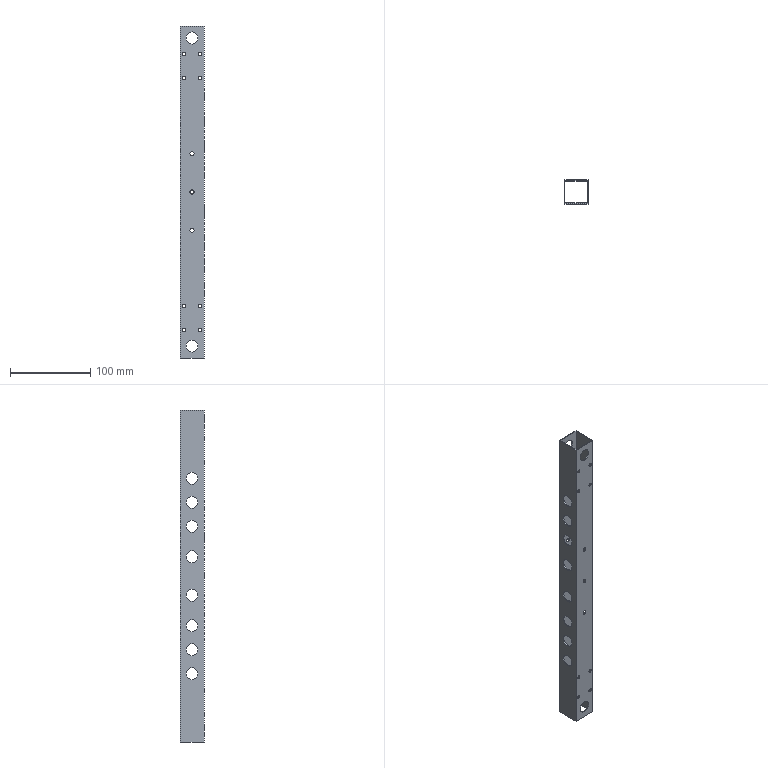Part | SolidWorks | features ICE 3, Extrusion 1, Shell 1 | 1 solid | 94 faces | box 30 x 30 x 415 mm | volume 44267 mm3 | cylinder 84 | plane 10 | commonest cylinder face diameters 15 x40 4.1 x32 5.2 x12